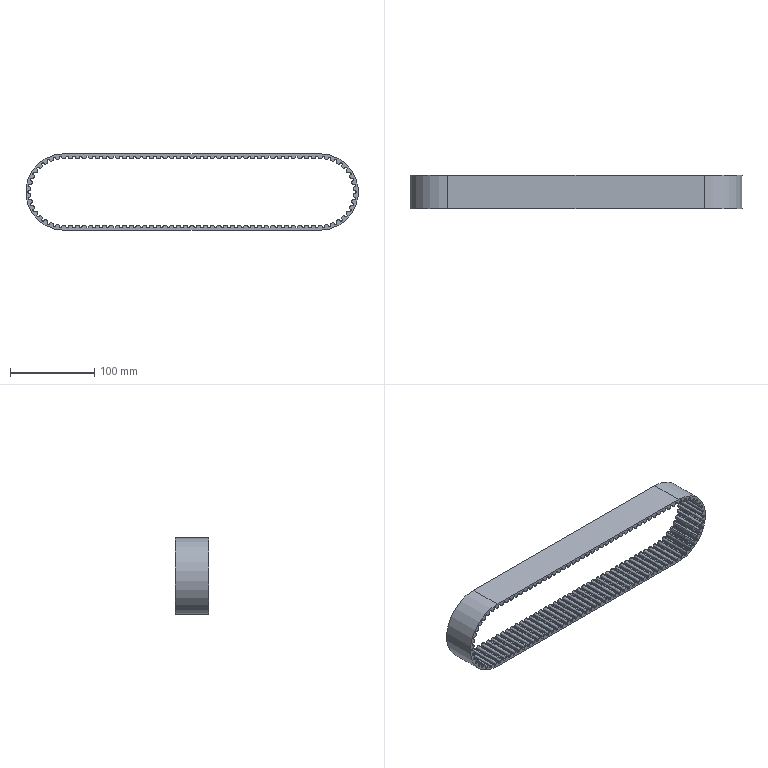Part | SolidWorks | features BaseBody 1 | 1 solid | 948 faces | box 394.448 x 40 x 90.448 mm | volume 157059 mm3 | plane 478 | cylinder 470 | commonest cylinder face diameters 1.5 x234 4.92 x234 90.448 x2